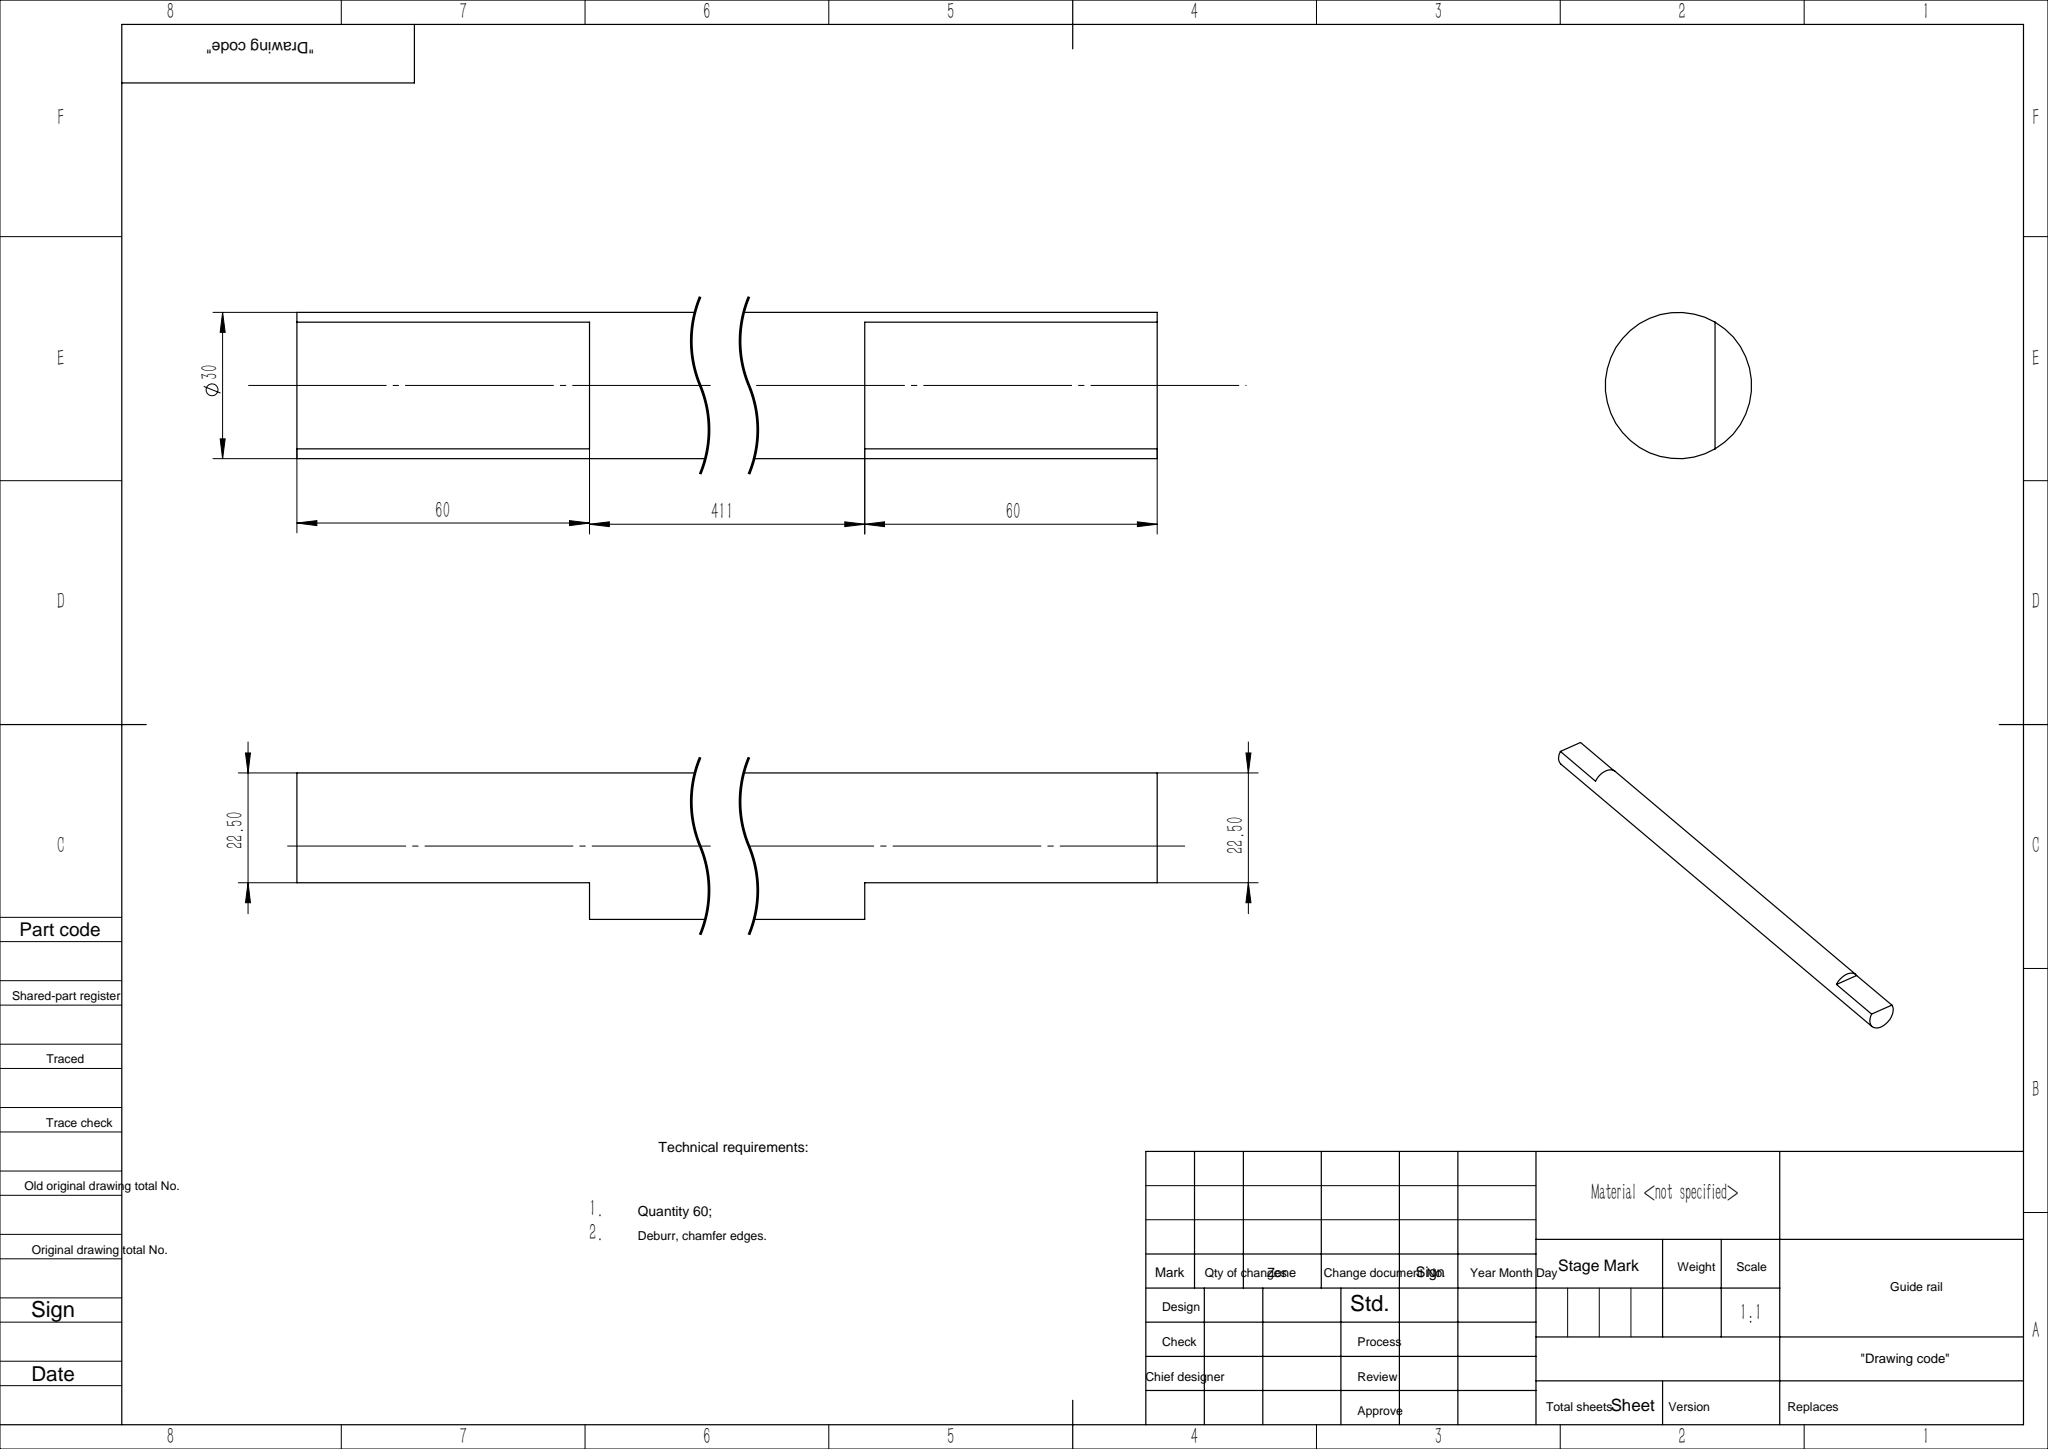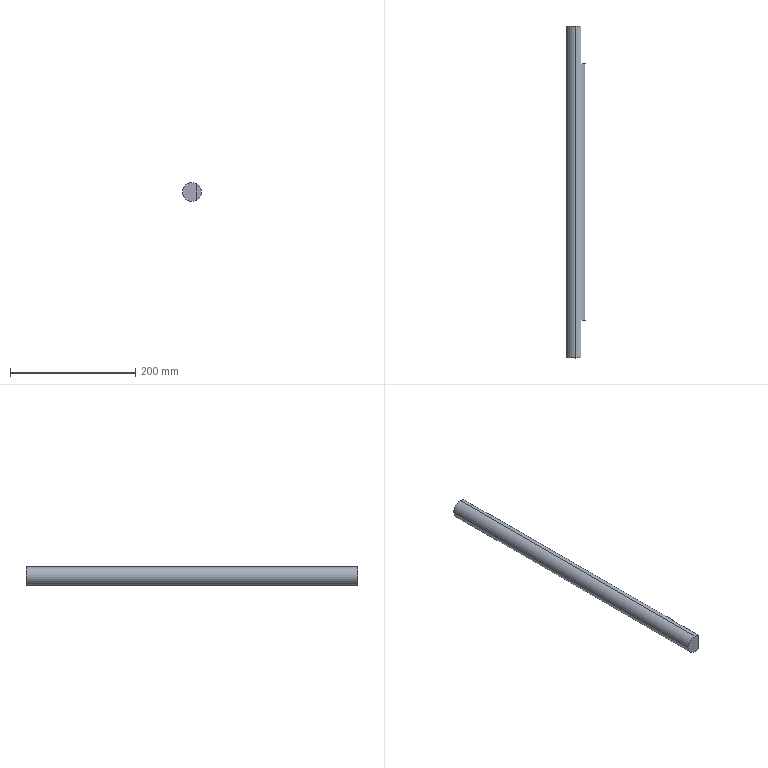Part | SolidWorks | features Extrusion 1, ICE 1, MirrorPattern 1 | 1 solid | 8 faces | box 30 x 531 x 30 mm | volume 358759 mm3 | plane 6 | cylinder 2 | commonest cylinder face diameters 30 x2
STEP:
#1=CARTESIAN_POINT('',(0.,531.,15.));
#2=VERTEX_POINT('',#1);
#3=CARTESIAN_POINT('',(7.5,531.,12.99));
#4=VERTEX_POINT('',#3);
#5=CARTESIAN_POINT('',(0.,531.,0.));
#6=DIRECTION('',(0.,1.,0.));
#7=DIRECTION('',(0.,0.,1.));
#8=AXIS2_PLACEMENT_3D('',#5,#6,#7);
#9=CIRCLE('',#8,15.);
#10=EDGE_CURVE('',#2,#4,#9,.T.);
#11=ORIENTED_EDGE('',*,*,#10,.F.);
#12=CARTESIAN_POINT('',(0.,0.,15.));
#13=VERTEX_POINT('',#12);
#14=CARTESIAN_POINT('',(0.,531.,15.));
#15=DIRECTION('',(0.,-1.,0.));
#16=VECTOR('',#15,1000.);
#17=LINE('',#14,#16);
#18=EDGE_CURVE('',#2,#13,#17,.T.);
#19=ORIENTED_EDGE('',*,*,#18,.T.);
#20=CARTESIAN_POINT('',(7.5,0.,12.99));
#21=VERTEX_POINT('',#20);
#22=CARTESIAN_POINT('',(0.,0.,0.));
#23=DIRECTION('',(0.,1.,0.));
#24=DIRECTION('',(0.,0.,1.));
#25=AXIS2_PLACEMENT_3D('',#22,#23,#24);
#26=CIRCLE('',#25,15.);
#27=EDGE_CURVE('',#13,#21,#26,.T.);
#28=ORIENTED_EDGE('',*,*,#27,.T.);
#29=CARTESIAN_POINT('',(7.5,60.,12.99));
#30=VERTEX_POINT('',#29);
#31=CARTESIAN_POINT('',(7.5,60.,12.99));
#32=DIRECTION('',(0.,-1.,0.));
#33=VECTOR('',#32,1000.);
#34=LINE('',#31,#33);
#35=EDGE_CURVE('',#30,#21,#34,.T.);
#36=ORIENTED_EDGE('',*,*,#35,.F.);
#37=CARTESIAN_POINT('',(7.5,60.,-12.99));
#38=VERTEX_POINT('',#37);
#39=CARTESIAN_POINT('',(0.,60.,0.));
#40=DIRECTION('',(0.,1.,0.));
#41=DIRECTION('',(0.,0.,1.));
#42=AXIS2_PLACEMENT_3D('',#39,#40,#41);
#43=CIRCLE('',#42,15.);
#44=EDGE_CURVE('',#30,#38,#43,.T.);
#45=ORIENTED_EDGE('',*,*,#44,.T.);
#46=CARTESIAN_POINT('',(7.5,0.,-12.99));
#47=VERTEX_POINT('',#46);
#48=CARTESIAN_POINT('',(7.5,60.,-12.99));
#49=DIRECTION('',(0.,-1.,0.));
#50=VECTOR('',#49,1000.);
#51=LINE('',#48,#50);
#52=EDGE_CURVE('',#38,#47,#51,.T.);
#53=ORIENTED_EDGE('',*,*,#52,.T.);
#54=CARTESIAN_POINT('',(0.,0.,-15.));
#55=VERTEX_POINT('',#54);
#56=CARTESIAN_POINT('',(0.,0.,0.));
#57=DIRECTION('',(0.,1.,0.));
#58=DIRECTION('',(0.,0.,1.));
#59=AXIS2_PLACEMENT_3D('',#56,#57,#58);
#60=CIRCLE('',#59,15.);
#61=EDGE_CURVE('',#47,#55,#60,.T.);
#62=ORIENTED_EDGE('',*,*,#61,.T.);
#63=CARTESIAN_POINT('',(0.,531.,-15.));
#64=VERTEX_POINT('',#63);
#65=CARTESIAN_POINT('',(0.,531.,-15.));
#66=DIRECTION('',(0.,-1.,0.));
#67=VECTOR('',#66,1000.);
#68=LINE('',#65,#67);
#69=EDGE_CURVE('',#64,#55,#68,.T.);
#70=ORIENTED_EDGE('',*,*,#69,.F.);
#71=CARTESIAN_POINT('',(7.5,531.,-12.99));
#72=VERTEX_POINT('',#71);
#73=CARTESIAN_POINT('',(0.,531.,0.));
#74=DIRECTION('',(0.,1.,0.));
#75=DIRECTION('',(0.,0.,1.));
#76=AXIS2_PLACEMENT_3D('',#73,#74,#75);
#77=CIRCLE('',#76,15.);
#78=EDGE_CURVE('',#72,#64,#77,.T.);
#79=ORIENTED_EDGE('',*,*,#78,.F.);
#80=CARTESIAN_POINT('',(7.5,471.,-12.99));
#81=VERTEX_POINT('',#80);
#82=CARTESIAN_POINT('',(7.5,471.,-12.99));
#83=DIRECTION('',(0.,1.,0.));
#84=VECTOR('',#83,1000.);
#85=LINE('',#82,#84);
#86=EDGE_CURVE('',#81,#72,#85,.T.);
#87=ORIENTED_EDGE('',*,*,#86,.F.);
#88=CARTESIAN_POINT('',(7.5,471.,12.99));
#89=VERTEX_POINT('',#88);
#90=CARTESIAN_POINT('',(0.,471.,0.));
#91=DIRECTION('',(0.,1.,0.));
#92=DIRECTION('',(0.,0.,1.));
#93=AXIS2_PLACEMENT_3D('',#90,#91,#92);
#94=CIRCLE('',#93,15.);
#95=EDGE_CURVE('',#89,#81,#94,.T.);
#96=ORIENTED_EDGE('',*,*,#95,.F.);
#97=CARTESIAN_POINT('',(7.5,471.,12.99));
#98=DIRECTION('',(0.,1.,0.));
#99=VECTOR('',#98,1000.);
#100=LINE('',#97,#99);
#101=EDGE_CURVE('',#89,#4,#100,.T.);
#102=ORIENTED_EDGE('',*,*,#101,.T.);
#103=EDGE_LOOP('',(#11,#19,#28,#36,#45,#53,#62,#70,#79,#87,#96,#102));
#104=FACE_OUTER_BOUND('',#103,.T.);
#105=CARTESIAN_POINT('',(0.,531.,0.));
#106=DIRECTION('',(0.,-1.,0.));
#107=DIRECTION('',(0.,0.,-1.));
#108=AXIS2_PLACEMENT_3D('',#105,#106,#107);
#109=CYLINDRICAL_SURFACE('',#108,15.);
#110=ADVANCED_FACE('',(#104),#109,.T.);
#111=ORIENTED_EDGE('',*,*,#18,.F.);
#112=CARTESIAN_POINT('',(0.,531.,0.));
#113=DIRECTION('',(0.,1.,0.));
#114=DIRECTION('',(0.,0.,1.));
#115=AXIS2_PLACEMENT_3D('',#112,#113,#114);
#116=CIRCLE('',#115,15.);
#117=EDGE_CURVE('',#64,#2,#116,.T.);
#118=ORIENTED_EDGE('',*,*,#117,.F.);
#119=ORIENTED_EDGE('',*,*,#69,.T.);
#120=CARTESIAN_POINT('',(0.,0.,0.));
#121=DIRECTION('',(0.,1.,0.));
#122=DIRECTION('',(0.,0.,1.));
#123=AXIS2_PLACEMENT_3D('',#120,#121,#122);
#124=CIRCLE('',#123,15.);
#125=EDGE_CURVE('',#55,#13,#124,.T.);
#126=ORIENTED_EDGE('',*,*,#125,.T.);
#127=EDGE_LOOP('',(#111,#118,#119,#126));
#128=FACE_OUTER_BOUND('',#127,.T.);
#129=CARTESIAN_POINT('',(0.,531.,0.));
#130=DIRECTION('',(0.,-1.,0.));
#131=DIRECTION('',(0.,0.,-1.));
#132=AXIS2_PLACEMENT_3D('',#129,#130,#131);
#133=CYLINDRICAL_SURFACE('',#132,15.);
#134=ADVANCED_FACE('',(#128),#133,.T.);
#135=CARTESIAN_POINT('',(7.5,0.,-12.99));
#136=DIRECTION('',(0.,0.,1.));
#137=VECTOR('',#136,1000.);
#138=LINE('',#135,#137);
#139=EDGE_CURVE('',#47,#21,#138,.T.);
#140=ORIENTED_EDGE('',*,*,#139,.T.);
#141=ORIENTED_EDGE('',*,*,#27,.F.);
#142=ORIENTED_EDGE('',*,*,#125,.F.);
#143=ORIENTED_EDGE('',*,*,#61,.F.);
#144=EDGE_LOOP('',(#140,#141,#142,#143));
#145=FACE_OUTER_BOUND('',#144,.T.);
#146=CARTESIAN_POINT('',(0.,0.,0.));
#147=DIRECTION('',(0.,1.,0.));
#148=DIRECTION('',(0.,0.,1.));
#149=AXIS2_PLACEMENT_3D('',#146,#147,#148);
#150=PLANE('',#149);
#151=ADVANCED_FACE('',(#145),#150,.F.);
#152=CARTESIAN_POINT('',(7.5,531.,-12.99));
#153=DIRECTION('',(0.,0.,1.));
#154=VECTOR('',#153,1000.);
#155=LINE('',#152,#154);
#156=EDGE_CURVE('',#72,#4,#155,.T.);
#157=ORIENTED_EDGE('',*,*,#156,.F.);
#158=ORIENTED_EDGE('',*,*,#78,.T.);
#159=ORIENTED_EDGE('',*,*,#117,.T.);
#160=ORIENTED_EDGE('',*,*,#10,.T.);
#161=EDGE_LOOP('',(#157,#158,#159,#160));
#162=FACE_OUTER_BOUND('',#161,.T.);
#163=CARTESIAN_POINT('',(0.,531.,0.));
#164=DIRECTION('',(0.,1.,0.));
#165=DIRECTION('',(0.,0.,1.));
#166=AXIS2_PLACEMENT_3D('',#163,#164,#165);
#167=PLANE('',#166);
#168=ADVANCED_FACE('',(#162),#167,.T.);
#169=ORIENTED_EDGE('',*,*,#156,.T.);
#170=ORIENTED_EDGE('',*,*,#101,.F.);
#171=CARTESIAN_POINT('',(7.5,471.,-12.99));
#172=DIRECTION('',(0.,0.,1.));
#173=VECTOR('',#172,1000.);
#174=LINE('',#171,#173);
#175=EDGE_CURVE('',#81,#89,#174,.T.);
#176=ORIENTED_EDGE('',*,*,#175,.F.);
#177=ORIENTED_EDGE('',*,*,#86,.T.);
#178=EDGE_LOOP('',(#169,#170,#176,#177));
#179=FACE_OUTER_BOUND('',#178,.T.);
#180=CARTESIAN_POINT('',(7.5,471.,-12.99));
#181=DIRECTION('',(-1.,0.,0.));
#182=DIRECTION('',(0.,0.,1.));
#183=AXIS2_PLACEMENT_3D('',#180,#181,#182);
#184=PLANE('',#183);
#185=ADVANCED_FACE('',(#179),#184,.F.);
#186=ORIENTED_EDGE('',*,*,#95,.T.);
#187=ORIENTED_EDGE('',*,*,#175,.T.);
#188=EDGE_LOOP('',(#186,#187));
#189=FACE_OUTER_BOUND('',#188,.T.);
#190=CARTESIAN_POINT('',(0.,471.,0.));
#191=DIRECTION('',(0.,1.,0.));
#192=DIRECTION('',(0.,0.,1.));
#193=AXIS2_PLACEMENT_3D('',#190,#191,#192);
#194=PLANE('',#193);
#195=ADVANCED_FACE('',(#189),#194,.T.);
#196=ORIENTED_EDGE('',*,*,#139,.F.);
#197=ORIENTED_EDGE('',*,*,#52,.F.);
#198=CARTESIAN_POINT('',(7.5,60.,-12.99));
#199=DIRECTION('',(0.,0.,1.));
#200=VECTOR('',#199,1000.);
#201=LINE('',#198,#200);
#202=EDGE_CURVE('',#38,#30,#201,.T.);
#203=ORIENTED_EDGE('',*,*,#202,.T.);
#204=ORIENTED_EDGE('',*,*,#35,.T.);
#205=EDGE_LOOP('',(#196,#197,#203,#204));
#206=FACE_OUTER_BOUND('',#205,.T.);
#207=CARTESIAN_POINT('',(7.5,60.,-12.99));
#208=DIRECTION('',(1.,0.,0.));
#209=DIRECTION('',(0.,0.,-1.));
#210=AXIS2_PLACEMENT_3D('',#207,#208,#209);
#211=PLANE('',#210);
#212=ADVANCED_FACE('',(#206),#211,.T.);
#213=ORIENTED_EDGE('',*,*,#44,.F.);
#214=ORIENTED_EDGE('',*,*,#202,.F.);
#215=EDGE_LOOP('',(#213,#214));
#216=FACE_OUTER_BOUND('',#215,.T.);
#217=CARTESIAN_POINT('',(0.,60.,0.));
#218=DIRECTION('',(0.,-1.,0.));
#219=DIRECTION('',(0.,0.,1.));
#220=AXIS2_PLACEMENT_3D('',#217,#218,#219);
#221=PLANE('',#220);
#222=ADVANCED_FACE('',(#216),#221,.T.);
#223=CLOSED_SHELL('',(#110,#134,#151,#168,#185,#195,#212,#222));
#224=MANIFOLD_SOLID_BREP('',#223);
#225=CARTESIAN_POINT('',(0.,0.,0.));
#226=DIRECTION('',(0.,0.,1.));
#227=DIRECTION('',(1.,0.,0.));
#228=AXIS2_PLACEMENT_3D('',#225,#226,#227);
#229=(LENGTH_UNIT()NAMED_UNIT(*)SI_UNIT(.MILLI.,.METRE.));
#230=UNCERTAINTY_MEASURE_WITH_UNIT(LENGTH_MEASURE(0.00001),#229,'','');
#231=(NAMED_UNIT(*)PLANE_ANGLE_UNIT()SI_UNIT($,.RADIAN.));
#232=(NAMED_UNIT(*)SI_UNIT($,.STERADIAN.)SOLID_ANGLE_UNIT());
#233=(GEOMETRIC_REPRESENTATION_CONTEXT(3)GLOBAL_UNCERTAINTY_ASSIGNED_CONTEXT((#230))GLOBAL_UNIT_ASSIGNED_CONTEXT((#229,#231,#232))REPRESENTATION_CONTEXT('',''));
#234=ADVANCED_BREP_SHAPE_REPRESENTATION('',(#224,#228),#233);